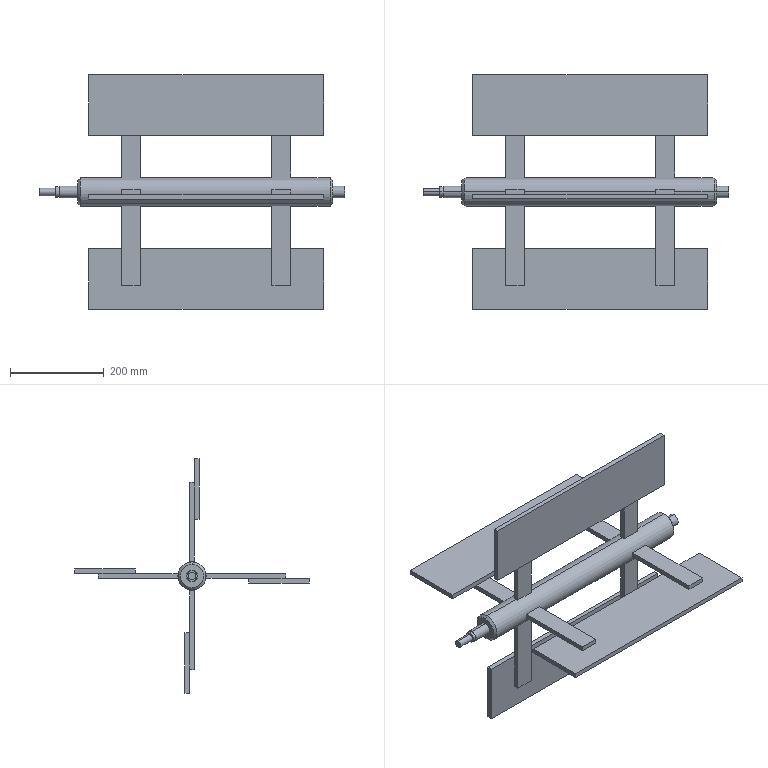Part | SolidWorks | features ICE 2, Chamfer 1, CirPattern 1, RefAxis 1, Revolution 1 | 1 solid | 84 faces | box 650 x 499.161 x 499.161 mm | volume 4694560 mm3 | plane 70 | cylinder 10 | cone 4 | commonest cylinder face diameters 25 x4 16 x2 22 x2 60 x2